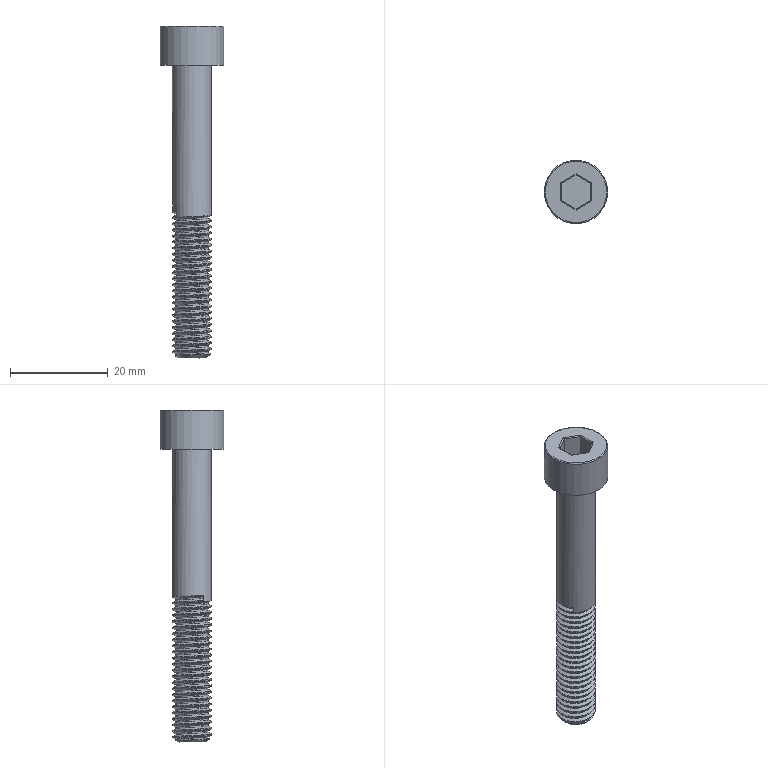Part | STEP file | Tube feed_id1162_x_t | 1 solid | 47 faces | box 13 x 13 x 68 mm | volume 3686 mm3 | cylinder 31 | plane 11 | cone 2 | spline 2 | torus 1 | commonest cylinder face diameters 8 x23 0.4 x6 6.75 x1 13 x1